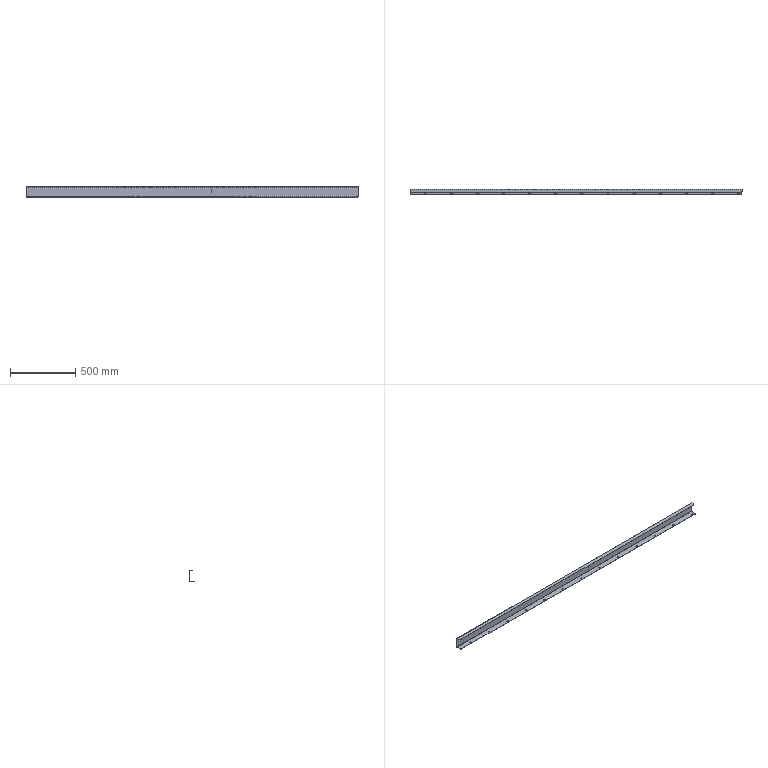Part | SolidWorks | features BaseBody 1 | 1 solid | 87 faces | box 2540 x 45 x 80 mm | volume 572600 mm3 | cylinder 51 | plane 36 | commonest cylinder face diameters 6 x39 4.2 x4 20 x4 1.473 x2 4.473 x2